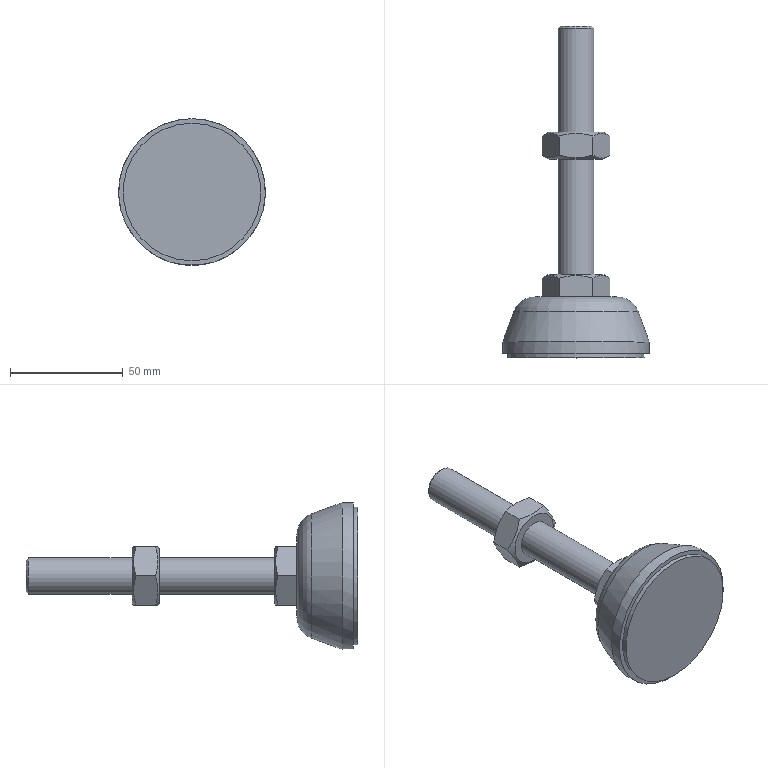Part | STEP file | Foot cup | 2 solids | 32 faces | box 65 x 147 x 65 mm | volume 56921 mm3 | plane 21 | cone 4 | cylinder 4 | torus 3 | commonest cylinder face diameters 16 x2 61 x1 65 x1
STEP:
#1=CARTESIAN_POINT('',(0.,96.,8.));
#2=VERTEX_POINT('',#1);
#3=CARTESIAN_POINT('',(0.,96.,0.));
#4=DIRECTION('',(0.,-1.,0.));
#5=DIRECTION('',(0.,0.,1.));
#6=AXIS2_PLACEMENT_3D('',#3,#4,#5);
#7=CIRCLE('',#6,8.);
#8=EDGE_CURVE('',#2,#2,#7,.T.);
#9=ORIENTED_EDGE('',*,*,#8,.F.);
#10=EDGE_LOOP('',(#9));
#11=FACE_BOUND('',#10,.T.);
#12=CARTESIAN_POINT('',(0.,96.,12.));
#13=VERTEX_POINT('',#12);
#14=CARTESIAN_POINT('',(0.,96.,0.));
#15=DIRECTION('',(0.,1.,0.));
#16=DIRECTION('',(0.,0.,1.));
#17=AXIS2_PLACEMENT_3D('',#14,#15,#16);
#18=CIRCLE('',#17,12.);
#19=EDGE_CURVE('',#13,#13,#18,.T.);
#20=ORIENTED_EDGE('',*,*,#19,.F.);
#21=EDGE_LOOP('',(#20));
#22=FACE_OUTER_BOUND('',#21,.T.);
#23=CARTESIAN_POINT('',(-15.,96.,0.));
#24=DIRECTION('',(0.,1.,0.));
#25=DIRECTION('',(0.,0.,1.));
#26=AXIS2_PLACEMENT_3D('',#23,#24,#25);
#27=PLANE('',#26);
#28=ADVANCED_FACE('',(#11,#22),#27,.F.);
#29=CARTESIAN_POINT('',(0.,45.,-8.));
#30=VERTEX_POINT('',#29);
#31=CARTESIAN_POINT('',(0.,45.,0.));
#32=DIRECTION('',(0.,1.,0.));
#33=DIRECTION('',(0.,0.,-1.));
#34=AXIS2_PLACEMENT_3D('',#31,#32,#33);
#35=CIRCLE('',#34,8.);
#36=EDGE_CURVE('',#30,#30,#35,.T.);
#37=ORIENTED_EDGE('',*,*,#36,.T.);
#38=EDGE_LOOP('',(#37));
#39=FACE_OUTER_BOUND('',#38,.T.);
#40=ORIENTED_EDGE('',*,*,#8,.T.);
#41=EDGE_LOOP('',(#40));
#42=FACE_OUTER_BOUND('',#41,.T.);
#43=CARTESIAN_POINT('',(0.,47.727,0.));
#44=DIRECTION('',(0.,1.,0.));
#45=DIRECTION('',(0.,0.,1.));
#46=AXIS2_PLACEMENT_3D('',#43,#44,#45);
#47=CYLINDRICAL_SURFACE('',#46,8.);
#48=ADVANCED_FACE('',(#39,#42),#47,.T.);
#49=CARTESIAN_POINT('',(0.,35.,18.177));
#50=VERTEX_POINT('',#49);
#51=CARTESIAN_POINT('',(0.,35.,0.));
#52=DIRECTION('',(0.,1.,0.));
#53=DIRECTION('',(0.,0.,1.));
#54=AXIS2_PLACEMENT_3D('',#51,#52,#53);
#55=CIRCLE('',#54,18.177);
#56=EDGE_CURVE('',#50,#50,#55,.T.);
#57=ORIENTED_EDGE('',*,*,#56,.T.);
#58=EDGE_LOOP('',(#57));
#59=FACE_OUTER_BOUND('',#58,.T.);
#60=CARTESIAN_POINT('',(-15.,35.,0.));
#61=VERTEX_POINT('',#60);
#62=CARTESIAN_POINT('',(-7.5,35.,12.99));
#63=VERTEX_POINT('',#62);
#64=CARTESIAN_POINT('',(-7.5,35.,12.99));
#65=DIRECTION('',(0.5,0.,0.866));
#66=VECTOR('',#65,1000.);
#67=LINE('',#64,#66);
#68=EDGE_CURVE('',#61,#63,#67,.T.);
#69=ORIENTED_EDGE('',*,*,#68,.F.);
#70=CARTESIAN_POINT('',(-7.5,35.,-12.99));
#71=VERTEX_POINT('',#70);
#72=CARTESIAN_POINT('',(-15.,35.,0.));
#73=DIRECTION('',(-0.5,0.,0.866));
#74=VECTOR('',#73,1000.);
#75=LINE('',#72,#74);
#76=EDGE_CURVE('',#71,#61,#75,.T.);
#77=ORIENTED_EDGE('',*,*,#76,.F.);
#78=CARTESIAN_POINT('',(7.5,35.,-12.99));
#79=VERTEX_POINT('',#78);
#80=CARTESIAN_POINT('',(-7.5,35.,-12.99));
#81=DIRECTION('',(-1.,0.,0.));
#82=VECTOR('',#81,1000.);
#83=LINE('',#80,#82);
#84=EDGE_CURVE('',#79,#71,#83,.T.);
#85=ORIENTED_EDGE('',*,*,#84,.F.);
#86=CARTESIAN_POINT('',(15.,35.,0.));
#87=VERTEX_POINT('',#86);
#88=CARTESIAN_POINT('',(7.5,35.,-12.99));
#89=DIRECTION('',(-0.5,0.,-0.866));
#90=VECTOR('',#89,1000.);
#91=LINE('',#88,#90);
#92=EDGE_CURVE('',#87,#79,#91,.T.);
#93=ORIENTED_EDGE('',*,*,#92,.F.);
#94=CARTESIAN_POINT('',(7.5,35.,12.99));
#95=VERTEX_POINT('',#94);
#96=CARTESIAN_POINT('',(15.,35.,0.));
#97=DIRECTION('',(0.5,0.,-0.866));
#98=VECTOR('',#97,1000.);
#99=LINE('',#96,#98);
#100=EDGE_CURVE('',#95,#87,#99,.T.);
#101=ORIENTED_EDGE('',*,*,#100,.F.);
#102=CARTESIAN_POINT('',(7.5,35.,12.99));
#103=DIRECTION('',(1.,0.,0.));
#104=VECTOR('',#103,1000.);
#105=LINE('',#102,#104);
#106=EDGE_CURVE('',#63,#95,#105,.T.);
#107=ORIENTED_EDGE('',*,*,#106,.F.);
#108=EDGE_LOOP('',(#69,#77,#85,#93,#101,#107));
#109=FACE_BOUND('',#108,.T.);
#110=CARTESIAN_POINT('',(-25.,35.,0.));
#111=DIRECTION('',(0.,1.,0.));
#112=DIRECTION('',(0.,0.,1.));
#113=AXIS2_PLACEMENT_3D('',#110,#111,#112);
#114=PLANE('',#113);
#115=ADVANCED_FACE('',(#59,#109),#114,.T.);
#116=CARTESIAN_POINT('',(0.,28.582,-27.513));
#117=VERTEX_POINT('',#116);
#118=CARTESIAN_POINT('',(0.,28.582,0.));
#119=DIRECTION('',(0.,-1.,0.));
#120=DIRECTION('',(0.,0.,-1.));
#121=AXIS2_PLACEMENT_3D('',#118,#119,#120);
#122=CIRCLE('',#121,27.513);
#123=EDGE_CURVE('',#117,#117,#122,.T.);
#124=ORIENTED_EDGE('',*,*,#123,.T.);
#125=EDGE_LOOP('',(#124));
#126=FACE_OUTER_BOUND('',#125,.T.);
#127=CARTESIAN_POINT('',(0.,15.,32.5));
#128=VERTEX_POINT('',#127);
#129=CARTESIAN_POINT('',(0.,15.,0.));
#130=DIRECTION('',(0.,1.,0.));
#131=DIRECTION('',(0.,0.,1.));
#132=AXIS2_PLACEMENT_3D('',#129,#130,#131);
#133=CIRCLE('',#132,32.5);
#134=EDGE_CURVE('',#128,#128,#133,.T.);
#135=ORIENTED_EDGE('',*,*,#134,.T.);
#136=EDGE_LOOP('',(#135));
#137=FACE_OUTER_BOUND('',#136,.T.);
#138=CARTESIAN_POINT('',(0.,-150.522,0.));
#139=DIRECTION('',(0.,1.,0.));
#140=DIRECTION('',(0.,0.,1.));
#141=AXIS2_PLACEMENT_3D('',#138,#139,#140);
#142=TOROIDAL_SURFACE('',#141,-439.308,500.);
#143=ADVANCED_FACE('',(#126,#137),#142,.T.);
#144=CARTESIAN_POINT('',(0.,10.,32.5));
#145=VERTEX_POINT('',#144);
#146=CARTESIAN_POINT('',(0.,10.,0.));
#147=DIRECTION('',(0.,1.,0.));
#148=DIRECTION('',(0.,0.,1.));
#149=AXIS2_PLACEMENT_3D('',#146,#147,#148);
#150=CIRCLE('',#149,32.5);
#151=EDGE_CURVE('',#145,#145,#150,.T.);
#152=ORIENTED_EDGE('',*,*,#151,.T.);
#153=EDGE_LOOP('',(#152));
#154=FACE_OUTER_BOUND('',#153,.T.);
#155=ORIENTED_EDGE('',*,*,#134,.F.);
#156=EDGE_LOOP('',(#155));
#157=FACE_OUTER_BOUND('',#156,.T.);
#158=CARTESIAN_POINT('',(0.,47.727,0.));
#159=DIRECTION('',(0.,1.,0.));
#160=DIRECTION('',(0.,0.,1.));
#161=AXIS2_PLACEMENT_3D('',#158,#159,#160);
#162=CYLINDRICAL_SURFACE('',#161,32.5);
#163=ADVANCED_FACE('',(#154,#157),#162,.T.);
#164=CARTESIAN_POINT('',(0.,10.,30.5));
#165=VERTEX_POINT('',#164);
#166=CARTESIAN_POINT('',(0.,10.,0.));
#167=DIRECTION('',(0.,1.,0.));
#168=DIRECTION('',(0.,0.,1.));
#169=AXIS2_PLACEMENT_3D('',#166,#167,#168);
#170=CIRCLE('',#169,30.5);
#171=EDGE_CURVE('',#165,#165,#170,.T.);
#172=ORIENTED_EDGE('',*,*,#171,.T.);
#173=EDGE_LOOP('',(#172));
#174=FACE_BOUND('',#173,.T.);
#175=ORIENTED_EDGE('',*,*,#151,.F.);
#176=EDGE_LOOP('',(#175));
#177=FACE_OUTER_BOUND('',#176,.T.);
#178=CARTESIAN_POINT('',(-30.5,10.,0.));
#179=DIRECTION('',(0.,-1.,0.));
#180=DIRECTION('',(0.,0.,-1.));
#181=AXIS2_PLACEMENT_3D('',#178,#179,#180);
#182=PLANE('',#181);
#183=ADVANCED_FACE('',(#174,#177),#182,.T.);
#184=CARTESIAN_POINT('',(0.,32.,22.398));
#185=VERTEX_POINT('',#184);
#186=CARTESIAN_POINT('',(0.,32.,0.));
#187=DIRECTION('',(0.,1.,0.));
#188=DIRECTION('',(0.,0.,1.));
#189=AXIS2_PLACEMENT_3D('',#186,#187,#188);
#190=CIRCLE('',#189,22.398);
#191=EDGE_CURVE('',#185,#185,#190,.T.);
#192=ORIENTED_EDGE('',*,*,#191,.T.);
#193=EDGE_LOOP('',(#192));
#194=FACE_OUTER_BOUND('',#193,.T.);
#195=ORIENTED_EDGE('',*,*,#171,.F.);
#196=EDGE_LOOP('',(#195));
#197=FACE_OUTER_BOUND('',#196,.T.);
#198=CARTESIAN_POINT('',(0.,-150.522,0.));
#199=DIRECTION('',(0.,1.,0.));
#200=DIRECTION('',(0.,0.,1.));
#201=AXIS2_PLACEMENT_3D('',#198,#199,#200);
#202=TOROIDAL_SURFACE('',#201,-439.308,496.474);
#203=ADVANCED_FACE('',(#194,#197),#202,.F.);
#204=ORIENTED_EDGE('',*,*,#191,.F.);
#205=EDGE_LOOP('',(#204));
#206=FACE_OUTER_BOUND('',#205,.T.);
#207=CARTESIAN_POINT('',(-22.398,32.,0.));
#208=DIRECTION('',(0.,-1.,0.));
#209=DIRECTION('',(0.,0.,-1.));
#210=AXIS2_PLACEMENT_3D('',#207,#208,#209);
#211=PLANE('',#210);
#212=ADVANCED_FACE('',(#206),#211,.T.);
#213=CARTESIAN_POINT('',(-15.,43.268,0.));
#214=VERTEX_POINT('',#213);
#215=CARTESIAN_POINT('',(-15.,45.,0.));
#216=DIRECTION('',(0.,-1.,0.));
#217=VECTOR('',#216,1000.);
#218=LINE('',#215,#217);
#219=EDGE_CURVE('',#214,#61,#218,.T.);
#220=ORIENTED_EDGE('',*,*,#219,.F.);
#221=CARTESIAN_POINT('',(-7.5,43.268,-12.99));
#222=VERTEX_POINT('',#221);
#223=CARTESIAN_POINT('',(-15.,43.268,0.));
#224=CARTESIAN_POINT('',(-14.388,43.621,-1.061));
#225=CARTESIAN_POINT('',(-13.771,43.913,-2.129));
#226=CARTESIAN_POINT('',(-12.525,44.316,-4.288));
#227=CARTESIAN_POINT('',(-11.895,44.427,-5.378));
#228=CARTESIAN_POINT('',(-10.938,44.429,-7.035));
#229=CARTESIAN_POINT('',(-10.618,44.401,-7.59));
#230=CARTESIAN_POINT('',(-9.984,44.296,-8.687));
#231=CARTESIAN_POINT('',(-9.67,44.217,-9.232));
#232=CARTESIAN_POINT('',(-8.731,43.914,-10.858));
#233=CARTESIAN_POINT('',(-8.113,43.622,-11.929));
#234=CARTESIAN_POINT('',(-7.5,43.268,-12.99));
#235=B_SPLINE_CURVE_WITH_KNOTS('',3,(#223,#224,#225,#226,#227,#228,#229,#230,#231,#232,#233,#234),.UNSPECIFIED.,.F.,.F.,(4,2,2,2,2,4),(0.000000238,0.003788,0.007575,0.009468,0.01136,0.01515),.UNSPECIFIED.);
#236=EDGE_CURVE('',#214,#222,#235,.T.);
#237=ORIENTED_EDGE('',*,*,#236,.T.);
#238=CARTESIAN_POINT('',(-7.5,45.,-12.99));
#239=DIRECTION('',(0.,-1.,0.));
#240=VECTOR('',#239,1000.);
#241=LINE('',#238,#240);
#242=EDGE_CURVE('',#222,#71,#241,.T.);
#243=ORIENTED_EDGE('',*,*,#242,.T.);
#244=ORIENTED_EDGE('',*,*,#76,.T.);
#245=EDGE_LOOP('',(#220,#237,#243,#244));
#246=FACE_OUTER_BOUND('',#245,.T.);
#247=CARTESIAN_POINT('',(-15.,45.,0.));
#248=DIRECTION('',(0.866,0.,0.5));
#249=DIRECTION('',(0.5,0.,-0.866));
#250=AXIS2_PLACEMENT_3D('',#247,#248,#249);
#251=PLANE('',#250);
#252=ADVANCED_FACE('',(#246),#251,.F.);
#253=CARTESIAN_POINT('',(-7.5,43.268,12.99));
#254=VERTEX_POINT('',#253);
#255=CARTESIAN_POINT('',(-7.5,45.,12.99));
#256=DIRECTION('',(0.,-1.,0.));
#257=VECTOR('',#256,1000.);
#258=LINE('',#255,#257);
#259=EDGE_CURVE('',#254,#63,#258,.T.);
#260=ORIENTED_EDGE('',*,*,#259,.F.);
#261=CARTESIAN_POINT('',(-7.5,43.268,12.99));
#262=CARTESIAN_POINT('',(-8.112,43.621,11.93));
#263=CARTESIAN_POINT('',(-8.729,43.913,10.862));
#264=CARTESIAN_POINT('',(-9.975,44.316,8.703));
#265=CARTESIAN_POINT('',(-10.605,44.427,7.612));
#266=CARTESIAN_POINT('',(-11.562,44.429,5.955));
#267=CARTESIAN_POINT('',(-11.882,44.401,5.401));
#268=CARTESIAN_POINT('',(-12.516,44.296,4.303));
#269=CARTESIAN_POINT('',(-12.83,44.217,3.758));
#270=CARTESIAN_POINT('',(-13.769,43.914,2.133));
#271=CARTESIAN_POINT('',(-14.387,43.622,1.062));
#272=CARTESIAN_POINT('',(-15.,43.268,0.));
#273=B_SPLINE_CURVE_WITH_KNOTS('',3,(#261,#262,#263,#264,#265,#266,#267,#268,#269,#270,#271,#272),.UNSPECIFIED.,.F.,.F.,(4,2,2,2,2,4),(0.000000238,0.003788,0.007575,0.009468,0.01136,0.01515),.UNSPECIFIED.);
#274=EDGE_CURVE('',#254,#214,#273,.T.);
#275=ORIENTED_EDGE('',*,*,#274,.T.);
#276=ORIENTED_EDGE('',*,*,#219,.T.);
#277=ORIENTED_EDGE('',*,*,#68,.T.);
#278=EDGE_LOOP('',(#260,#275,#276,#277));
#279=FACE_OUTER_BOUND('',#278,.T.);
#280=CARTESIAN_POINT('',(-7.5,45.,12.99));
#281=DIRECTION('',(0.866,0.,-0.5));
#282=DIRECTION('',(-0.5,0.,-0.866));
#283=AXIS2_PLACEMENT_3D('',#280,#281,#282);
#284=PLANE('',#283);
#285=ADVANCED_FACE('',(#279),#284,.F.);
#286=CARTESIAN_POINT('',(7.5,43.268,12.99));
#287=VERTEX_POINT('',#286);
#288=CARTESIAN_POINT('',(7.5,45.,12.99));
#289=DIRECTION('',(0.,-1.,0.));
#290=VECTOR('',#289,1000.);
#291=LINE('',#288,#290);
#292=EDGE_CURVE('',#287,#95,#291,.T.);
#293=ORIENTED_EDGE('',*,*,#292,.F.);
#294=CARTESIAN_POINT('',(7.5,43.268,12.99));
#295=CARTESIAN_POINT('',(6.288,43.618,12.99));
#296=CARTESIAN_POINT('',(5.059,43.909,12.99));
#297=CARTESIAN_POINT('',(3.181,44.214,12.99));
#298=CARTESIAN_POINT('',(2.547,44.294,12.99));
#299=CARTESIAN_POINT('',(1.272,44.401,12.99));
#300=CARTESIAN_POINT('',(0.6359,44.428,12.99));
#301=CARTESIAN_POINT('',(-1.265,44.428,12.99));
#302=CARTESIAN_POINT('',(-2.525,44.319,12.99));
#303=CARTESIAN_POINT('',(-4.404,44.017,12.99));
#304=CARTESIAN_POINT('',(-5.029,43.892,12.99));
#305=CARTESIAN_POINT('',(-6.275,43.606,12.99));
#306=CARTESIAN_POINT('',(-6.89,43.444,12.99));
#307=CARTESIAN_POINT('',(-7.5,43.268,12.99));
#308=B_SPLINE_CURVE_WITH_KNOTS('',3,(#294,#295,#296,#297,#298,#299,#300,#301,#302,#303,#304,#305,#306,#307),.UNSPECIFIED.,.F.,.F.,(4,2,2,2,2,2,4),(0.005592,0.009378,0.01127,0.01316,0.01695,0.01884,0.02073),.UNSPECIFIED.);
#309=EDGE_CURVE('',#287,#254,#308,.T.);
#310=ORIENTED_EDGE('',*,*,#309,.T.);
#311=ORIENTED_EDGE('',*,*,#259,.T.);
#312=ORIENTED_EDGE('',*,*,#106,.T.);
#313=EDGE_LOOP('',(#293,#310,#311,#312));
#314=FACE_OUTER_BOUND('',#313,.T.);
#315=CARTESIAN_POINT('',(7.5,45.,12.99));
#316=DIRECTION('',(0.,0.,-1.));
#317=DIRECTION('',(-1.,0.,0.));
#318=AXIS2_PLACEMENT_3D('',#315,#316,#317);
#319=PLANE('',#318);
#320=ADVANCED_FACE('',(#314),#319,.F.);
#321=CARTESIAN_POINT('',(15.,43.268,0.));
#322=VERTEX_POINT('',#321);
#323=CARTESIAN_POINT('',(15.,45.,0.));
#324=DIRECTION('',(0.,-1.,0.));
#325=VECTOR('',#324,1000.);
#326=LINE('',#323,#325);
#327=EDGE_CURVE('',#322,#87,#326,.T.);
#328=ORIENTED_EDGE('',*,*,#327,.F.);
#329=CARTESIAN_POINT('',(15.,43.268,0.));
#330=CARTESIAN_POINT('',(14.388,43.621,1.061));
#331=CARTESIAN_POINT('',(13.771,43.913,2.129));
#332=CARTESIAN_POINT('',(12.525,44.316,4.288));
#333=CARTESIAN_POINT('',(11.895,44.427,5.378));
#334=CARTESIAN_POINT('',(10.938,44.429,7.035));
#335=CARTESIAN_POINT('',(10.618,44.401,7.59));
#336=CARTESIAN_POINT('',(9.984,44.296,8.687));
#337=CARTESIAN_POINT('',(9.67,44.217,9.232));
#338=CARTESIAN_POINT('',(8.731,43.914,10.858));
#339=CARTESIAN_POINT('',(8.113,43.622,11.929));
#340=CARTESIAN_POINT('',(7.5,43.268,12.99));
#341=B_SPLINE_CURVE_WITH_KNOTS('',3,(#329,#330,#331,#332,#333,#334,#335,#336,#337,#338,#339,#340),.UNSPECIFIED.,.F.,.F.,(4,2,2,2,2,4),(0.000000238,0.003788,0.007575,0.009468,0.01136,0.01515),.UNSPECIFIED.);
#342=EDGE_CURVE('',#322,#287,#341,.T.);
#343=ORIENTED_EDGE('',*,*,#342,.T.);
#344=ORIENTED_EDGE('',*,*,#292,.T.);
#345=ORIENTED_EDGE('',*,*,#100,.T.);
#346=EDGE_LOOP('',(#328,#343,#344,#345));
#347=FACE_OUTER_BOUND('',#346,.T.);
#348=CARTESIAN_POINT('',(15.,45.,0.));
#349=DIRECTION('',(-0.866,0.,-0.5));
#350=DIRECTION('',(-0.5,0.,0.866));
#351=AXIS2_PLACEMENT_3D('',#348,#349,#350);
#352=PLANE('',#351);
#353=ADVANCED_FACE('',(#347),#352,.F.);
#354=CARTESIAN_POINT('',(7.5,43.268,-12.99));
#355=VERTEX_POINT('',#354);
#356=CARTESIAN_POINT('',(7.5,45.,-12.99));
#357=DIRECTION('',(0.,-1.,0.));
#358=VECTOR('',#357,1000.);
#359=LINE('',#356,#358);
#360=EDGE_CURVE('',#355,#79,#359,.T.);
#361=ORIENTED_EDGE('',*,*,#360,.F.);
#362=CARTESIAN_POINT('',(7.5,43.268,-12.99));
#363=CARTESIAN_POINT('',(8.112,43.621,-11.93));
#364=CARTESIAN_POINT('',(8.729,43.913,-10.862));
#365=CARTESIAN_POINT('',(9.975,44.316,-8.703));
#366=CARTESIAN_POINT('',(10.605,44.427,-7.612));
#367=CARTESIAN_POINT('',(11.562,44.429,-5.955));
#368=CARTESIAN_POINT('',(11.882,44.401,-5.401));
#369=CARTESIAN_POINT('',(12.516,44.296,-4.303));
#370=CARTESIAN_POINT('',(12.83,44.217,-3.758));
#371=CARTESIAN_POINT('',(13.769,43.914,-2.133));
#372=CARTESIAN_POINT('',(14.387,43.622,-1.062));
#373=CARTESIAN_POINT('',(15.,43.268,0.));
#374=B_SPLINE_CURVE_WITH_KNOTS('',3,(#362,#363,#364,#365,#366,#367,#368,#369,#370,#371,#372,#373),.UNSPECIFIED.,.F.,.F.,(4,2,2,2,2,4),(0.000000238,0.003788,0.007575,0.009468,0.01136,0.01515),.UNSPECIFIED.);
#375=EDGE_CURVE('',#355,#322,#374,.T.);
#376=ORIENTED_EDGE('',*,*,#375,.T.);
#377=ORIENTED_EDGE('',*,*,#327,.T.);
#378=ORIENTED_EDGE('',*,*,#92,.T.);
#379=EDGE_LOOP('',(#361,#376,#377,#378));
#380=FACE_OUTER_BOUND('',#379,.T.);
#381=CARTESIAN_POINT('',(7.5,45.,-12.99));
#382=DIRECTION('',(-0.866,0.,0.5));
#383=DIRECTION('',(0.5,0.,0.866));
#384=AXIS2_PLACEMENT_3D('',#381,#382,#383);
#385=PLANE('',#384);
#386=ADVANCED_FACE('',(#380),#385,.F.);
#387=ORIENTED_EDGE('',*,*,#242,.F.);
#388=CARTESIAN_POINT('',(-7.5,43.268,-12.99));
#389=CARTESIAN_POINT('',(-6.89,43.444,-12.99));
#390=CARTESIAN_POINT('',(-6.275,43.606,-12.99));
#391=CARTESIAN_POINT('',(-5.029,43.892,-12.99));
#392=CARTESIAN_POINT('',(-4.404,44.017,-12.99));
#393=CARTESIAN_POINT('',(-2.525,44.319,-12.99));
#394=CARTESIAN_POINT('',(-1.265,44.428,-12.99));
#395=CARTESIAN_POINT('',(0.6359,44.428,-12.99));
#396=CARTESIAN_POINT('',(1.272,44.401,-12.99));
#397=CARTESIAN_POINT('',(2.547,44.294,-12.99));
#398=CARTESIAN_POINT('',(3.181,44.214,-12.99));
#399=CARTESIAN_POINT('',(5.059,43.909,-12.99));
#400=CARTESIAN_POINT('',(6.288,43.618,-12.99));
#401=CARTESIAN_POINT('',(7.5,43.268,-12.99));
#402=B_SPLINE_CURVE_WITH_KNOTS('',3,(#388,#389,#390,#391,#392,#393,#394,#395,#396,#397,#398,#399,#400,#401),.UNSPECIFIED.,.F.,.F.,(4,2,2,2,2,2,4),(0.01329,0.01519,0.01709,0.02088,0.02278,0.02468,0.02847),.UNSPECIFIED.);
#403=EDGE_CURVE('',#222,#355,#402,.T.);
#404=ORIENTED_EDGE('',*,*,#403,.T.);
#405=ORIENTED_EDGE('',*,*,#360,.T.);
#406=ORIENTED_EDGE('',*,*,#84,.T.);
#407=EDGE_LOOP('',(#387,#404,#405,#406));
#408=FACE_OUTER_BOUND('',#407,.T.);
#409=CARTESIAN_POINT('',(-7.5,45.,-12.99));
#410=DIRECTION('',(0.,0.,1.));
#411=DIRECTION('',(1.,0.,0.));
#412=AXIS2_PLACEMENT_3D('',#409,#410,#411);
#413=PLANE('',#412);
#414=ADVANCED_FACE('',(#408),#413,.F.);
#415=CARTESIAN_POINT('',(0.,45.,-12.));
#416=VERTEX_POINT('',#415);
#417=CARTESIAN_POINT('',(0.,45.,0.));
#418=DIRECTION('',(0.,-1.,0.));
#419=DIRECTION('',(0.,0.,-1.));
#420=AXIS2_PLACEMENT_3D('',#417,#418,#419);
#421=CIRCLE('',#420,12.);
#422=EDGE_CURVE('',#416,#416,#421,.T.);
#423=ORIENTED_EDGE('',*,*,#422,.T.);
#424=EDGE_LOOP('',(#423));
#425=FACE_BOUND('',#424,.T.);
#426=ORIENTED_EDGE('',*,*,#274,.F.);
#427=ORIENTED_EDGE('',*,*,#309,.F.);
#428=ORIENTED_EDGE('',*,*,#342,.F.);
#429=ORIENTED_EDGE('',*,*,#375,.F.);
#430=ORIENTED_EDGE('',*,*,#403,.F.);
#431=ORIENTED_EDGE('',*,*,#236,.F.);
#432=EDGE_LOOP('',(#426,#427,#428,#429,#430,#431));
#433=FACE_OUTER_BOUND('',#432,.T.);
#434=CARTESIAN_POINT('',(0.,45.,0.));
#435=DIRECTION('',(0.,-1.,0.));
#436=DIRECTION('',(0.,0.,-1.));
#437=AXIS2_PLACEMENT_3D('',#434,#435,#436);
#438=CONICAL_SURFACE('',#437,12.,1.047);
#439=ADVANCED_FACE('',(#425,#433),#438,.T.);
#440=ORIENTED_EDGE('',*,*,#422,.F.);
#441=EDGE_LOOP('',(#440));
#442=FACE_OUTER_BOUND('',#441,.T.);
#443=ORIENTED_EDGE('',*,*,#36,.F.);
#444=EDGE_LOOP('',(#443));
#445=FACE_BOUND('',#444,.T.);
#446=CARTESIAN_POINT('',(0.,45.,-25.981));
#447=DIRECTION('',(0.,-1.,0.));
#448=DIRECTION('',(0.,0.,-1.));
#449=AXIS2_PLACEMENT_3D('',#446,#447,#448);
#450=PLANE('',#449);
#451=ADVANCED_FACE('',(#442,#445),#450,.F.);
#452=ORIENTED_EDGE('',*,*,#19,.T.);
#453=EDGE_LOOP('',(#452));
#454=FACE_BOUND('',#453,.T.);
#455=CARTESIAN_POINT('',(-15.,97.732,0.));
#456=VERTEX_POINT('',#455);
#457=CARTESIAN_POINT('',(-7.5,97.732,-12.99));
#458=VERTEX_POINT('',#457);
#459=CARTESIAN_POINT('',(-15.,97.732,0.));
#460=CARTESIAN_POINT('',(-14.388,97.379,-1.061));
#461=CARTESIAN_POINT('',(-13.771,97.087,-2.129));
#462=CARTESIAN_POINT('',(-12.525,96.684,-4.288));
#463=CARTESIAN_POINT('',(-11.895,96.573,-5.378));
#464=CARTESIAN_POINT('',(-10.938,96.571,-7.035));
#465=CARTESIAN_POINT('',(-10.618,96.599,-7.59));
#466=CARTESIAN_POINT('',(-9.984,96.704,-8.687));
#467=CARTESIAN_POINT('',(-9.67,96.783,-9.232));
#468=CARTESIAN_POINT('',(-8.731,97.086,-10.858));
#469=CARTESIAN_POINT('',(-8.113,97.378,-11.929));
#470=CARTESIAN_POINT('',(-7.5,97.732,-12.99));
#471=B_SPLINE_CURVE_WITH_KNOTS('',3,(#459,#460,#461,#462,#463,#464,#465,#466,#467,#468,#469,#470),.UNSPECIFIED.,.F.,.F.,(4,2,2,2,2,4),(0.000000238,0.003788,0.007575,0.009468,0.01136,0.01515),.UNSPECIFIED.);
#472=EDGE_CURVE('',#456,#458,#471,.T.);
#473=ORIENTED_EDGE('',*,*,#472,.T.);
#474=CARTESIAN_POINT('',(7.5,97.732,-12.99));
#475=VERTEX_POINT('',#474);
#476=CARTESIAN_POINT('',(-7.5,97.732,-12.99));
#477=CARTESIAN_POINT('',(-6.89,97.556,-12.99));
#478=CARTESIAN_POINT('',(-6.275,97.394,-12.99));
#479=CARTESIAN_POINT('',(-5.029,97.108,-12.99));
#480=CARTESIAN_POINT('',(-4.404,96.983,-12.99));
#481=CARTESIAN_POINT('',(-2.525,96.681,-12.99));
#482=CARTESIAN_POINT('',(-1.265,96.572,-12.99));
#483=CARTESIAN_POINT('',(0.6359,96.572,-12.99));
#484=CARTESIAN_POINT('',(1.272,96.599,-12.99));
#485=CARTESIAN_POINT('',(2.547,96.706,-12.99));
#486=CARTESIAN_POINT('',(3.181,96.786,-12.99));
#487=CARTESIAN_POINT('',(5.059,97.091,-12.99));
#488=CARTESIAN_POINT('',(6.288,97.382,-12.99));
#489=CARTESIAN_POINT('',(7.5,97.732,-12.99));
#490=B_SPLINE_CURVE_WITH_KNOTS('',3,(#476,#477,#478,#479,#480,#481,#482,#483,#484,#485,#486,#487,#488,#489),.UNSPECIFIED.,.F.,.F.,(4,2,2,2,2,2,4),(0.01329,0.01519,0.01709,0.02088,0.02278,0.02468,0.02847),.UNSPECIFIED.);
#491=EDGE_CURVE('',#458,#475,#490,.T.);
#492=ORIENTED_EDGE('',*,*,#491,.T.);
#493=CARTESIAN_POINT('',(15.,97.732,0.));
#494=VERTEX_POINT('',#493);
#495=CARTESIAN_POINT('',(7.5,97.732,-12.99));
#496=CARTESIAN_POINT('',(8.112,97.379,-11.93));
#497=CARTESIAN_POINT('',(8.729,97.087,-10.862));
#498=CARTESIAN_POINT('',(9.975,96.684,-8.703));
#499=CARTESIAN_POINT('',(10.605,96.573,-7.612));
#500=CARTESIAN_POINT('',(11.562,96.571,-5.955));
#501=CARTESIAN_POINT('',(11.882,96.599,-5.401));
#502=CARTESIAN_POINT('',(12.516,96.704,-4.303));
#503=CARTESIAN_POINT('',(12.83,96.783,-3.758));
#504=CARTESIAN_POINT('',(13.769,97.086,-2.133));
#505=CARTESIAN_POINT('',(14.387,97.378,-1.062));
#506=CARTESIAN_POINT('',(15.,97.732,0.));
#507=B_SPLINE_CURVE_WITH_KNOTS('',3,(#495,#496,#497,#498,#499,#500,#501,#502,#503,#504,#505,#506),.UNSPECIFIED.,.F.,.F.,(4,2,2,2,2,4),(0.000000238,0.003788,0.007575,0.009468,0.01136,0.01515),.UNSPECIFIED.);
#508=EDGE_CURVE('',#475,#494,#507,.T.);
#509=ORIENTED_EDGE('',*,*,#508,.T.);
#510=CARTESIAN_POINT('',(7.5,97.732,12.99));
#511=VERTEX_POINT('',#510);
#512=CARTESIAN_POINT('',(15.,97.732,0.));
#513=CARTESIAN_POINT('',(14.388,97.379,1.061));
#514=CARTESIAN_POINT('',(13.771,97.087,2.129));
#515=CARTESIAN_POINT('',(12.525,96.684,4.288));
#516=CARTESIAN_POINT('',(11.895,96.573,5.378));
#517=CARTESIAN_POINT('',(10.938,96.571,7.035));
#518=CARTESIAN_POINT('',(10.618,96.599,7.59));
#519=CARTESIAN_POINT('',(9.984,96.704,8.687));
#520=CARTESIAN_POINT('',(9.67,96.783,9.232));
#521=CARTESIAN_POINT('',(8.731,97.086,10.858));
#522=CARTESIAN_POINT('',(8.113,97.378,11.929));
#523=CARTESIAN_POINT('',(7.5,97.732,12.99));
#524=B_SPLINE_CURVE_WITH_KNOTS('',3,(#512,#513,#514,#515,#516,#517,#518,#519,#520,#521,#522,#523),.UNSPECIFIED.,.F.,.F.,(4,2,2,2,2,4),(0.000000238,0.003788,0.007575,0.009468,0.01136,0.01515),.UNSPECIFIED.);
#525=EDGE_CURVE('',#494,#511,#524,.T.);
#526=ORIENTED_EDGE('',*,*,#525,.T.);
#527=CARTESIAN_POINT('',(-7.5,97.732,12.99));
#528=VERTEX_POINT('',#527);
#529=CARTESIAN_POINT('',(7.5,97.732,12.99));
#530=CARTESIAN_POINT('',(6.288,97.382,12.99));
#531=CARTESIAN_POINT('',(5.059,97.091,12.99));
#532=CARTESIAN_POINT('',(3.181,96.786,12.99));
#533=CARTESIAN_POINT('',(2.547,96.706,12.99));
#534=CARTESIAN_POINT('',(1.272,96.599,12.99));
#535=CARTESIAN_POINT('',(0.6359,96.572,12.99));
#536=CARTESIAN_POINT('',(-1.265,96.572,12.99));
#537=CARTESIAN_POINT('',(-2.525,96.681,12.99));
#538=CARTESIAN_POINT('',(-4.404,96.983,12.99));
#539=CARTESIAN_POINT('',(-5.029,97.108,12.99));
#540=CARTESIAN_POINT('',(-6.275,97.394,12.99));
#541=CARTESIAN_POINT('',(-6.89,97.556,12.99));
#542=CARTESIAN_POINT('',(-7.5,97.732,12.99));
#543=B_SPLINE_CURVE_WITH_KNOTS('',3,(#529,#530,#531,#532,#533,#534,#535,#536,#537,#538,#539,#540,#541,#542),.UNSPECIFIED.,.F.,.F.,(4,2,2,2,2,2,4),(0.005592,0.009378,0.01127,0.01316,0.01695,0.01884,0.02073),.UNSPECIFIED.);
#544=EDGE_CURVE('',#511,#528,#543,.T.);
#545=ORIENTED_EDGE('',*,*,#544,.T.);
#546=CARTESIAN_POINT('',(-7.5,97.732,12.99));
#547=CARTESIAN_POINT('',(-8.112,97.379,11.93));
#548=CARTESIAN_POINT('',(-8.729,97.087,10.862));
#549=CARTESIAN_POINT('',(-9.975,96.684,8.703));
#550=CARTESIAN_POINT('',(-10.605,96.573,7.612));
#551=CARTESIAN_POINT('',(-11.562,96.571,5.955));
#552=CARTESIAN_POINT('',(-11.882,96.599,5.401));
#553=CARTESIAN_POINT('',(-12.516,96.704,4.303));
#554=CARTESIAN_POINT('',(-12.83,96.783,3.758));
#555=CARTESIAN_POINT('',(-13.769,97.086,2.133));
#556=CARTESIAN_POINT('',(-14.387,97.378,1.062));
#557=CARTESIAN_POINT('',(-15.,97.732,0.));
#558=B_SPLINE_CURVE_WITH_KNOTS('',3,(#546,#547,#548,#549,#550,#551,#552,#553,#554,#555,#556,#557),.UNSPECIFIED.,.F.,.F.,(4,2,2,2,2,4),(0.000000238,0.003788,0.007575,0.009468,0.01136,0.01515),.UNSPECIFIED.);
#559=EDGE_CURVE('',#528,#456,#558,.T.);
#560=ORIENTED_EDGE('',*,*,#559,.T.);
#561=EDGE_LOOP('',(#473,#492,#509,#526,#545,#560));
#562=FACE_OUTER_BOUND('',#561,.T.);
#563=CARTESIAN_POINT('',(0.,97.732,0.));
#564=DIRECTION('',(0.,1.,0.));
#565=DIRECTION('',(0.,0.,1.));
#566=AXIS2_PLACEMENT_3D('',#563,#564,#565);
#567=CONICAL_SURFACE('',#566,15.,1.047);
#568=ADVANCED_FACE('',(#454,#562),#567,.T.);
#569=CARTESIAN_POINT('',(0.,155.,7.));
#570=VERTEX_POINT('',#569);
#571=CARTESIAN_POINT('',(0.,155.,0.));
#572=DIRECTION('',(0.,1.,0.));
#573=DIRECTION('',(0.,0.,1.));
#574=AXIS2_PLACEMENT_3D('',#571,#572,#573);
#575=CIRCLE('',#574,7.);
#576=EDGE_CURVE('',#570,#570,#575,.T.);
#577=ORIENTED_EDGE('',*,*,#576,.T.);
#578=EDGE_LOOP('',(#577));
#579=FACE_OUTER_BOUND('',#578,.T.);
#580=CARTESIAN_POINT('',(-8.,155.,0.));
#581=DIRECTION('',(0.,1.,0.));
#582=DIRECTION('',(0.,0.,1.));
#583=AXIS2_PLACEMENT_3D('',#580,#581,#582);
#584=PLANE('',#583);
#585=ADVANCED_FACE('',(#579),#584,.T.);
#586=CARTESIAN_POINT('',(0.,154.,8.));
#587=VERTEX_POINT('',#586);
#588=CARTESIAN_POINT('',(0.,154.,0.));
#589=DIRECTION('',(0.,-1.,0.));
#590=DIRECTION('',(0.,0.,1.));
#591=AXIS2_PLACEMENT_3D('',#588,#589,#590);
#592=CIRCLE('',#591,8.);
#593=EDGE_CURVE('',#587,#587,#592,.T.);
#594=ORIENTED_EDGE('',*,*,#593,.F.);
#595=EDGE_LOOP('',(#594));
#596=FACE_OUTER_BOUND('',#595,.T.);
#597=ORIENTED_EDGE('',*,*,#576,.F.);
#598=EDGE_LOOP('',(#597));
#599=FACE_BOUND('',#598,.T.);
#600=CARTESIAN_POINT('',(0.,155.,0.));
#601=DIRECTION('',(0.,-1.,0.));
#602=DIRECTION('',(0.,0.,-1.));
#603=AXIS2_PLACEMENT_3D('',#600,#601,#602);
#604=CONICAL_SURFACE('',#603,7.,0.7854);
#605=ADVANCED_FACE('',(#596,#599),#604,.T.);
#606=CARTESIAN_POINT('',(0.,108.,8.));
#607=VERTEX_POINT('',#606);
#608=CARTESIAN_POINT('',(0.,108.,0.));
#609=DIRECTION('',(0.,-1.,0.));
#610=DIRECTION('',(0.,0.,1.));
#611=AXIS2_PLACEMENT_3D('',#608,#609,#610);
#612=CIRCLE('',#611,8.);
#613=EDGE_CURVE('',#607,#607,#612,.T.);
#614=ORIENTED_EDGE('',*,*,#613,.F.);
#615=EDGE_LOOP('',(#614));
#616=FACE_OUTER_BOUND('',#615,.T.);
#617=ORIENTED_EDGE('',*,*,#593,.T.);
#618=EDGE_LOOP('',(#617));
#619=FACE_OUTER_BOUND('',#618,.T.);
#620=CARTESIAN_POINT('',(0.,47.727,0.));
#621=DIRECTION('',(0.,1.,0.));
#622=DIRECTION('',(0.,0.,1.));
#623=AXIS2_PLACEMENT_3D('',#620,#621,#622);
#624=CYLINDRICAL_SURFACE('',#623,8.);
#625=ADVANCED_FACE('',(#616,#619),#624,.T.);
#626=ORIENTED_EDGE('',*,*,#613,.T.);
#627=EDGE_LOOP('',(#626));
#628=FACE_BOUND('',#627,.T.);
#629=CARTESIAN_POINT('',(0.,108.,12.));
#630=VERTEX_POINT('',#629);
#631=CARTESIAN_POINT('',(0.,108.,0.));
#632=DIRECTION('',(0.,1.,0.));
#633=DIRECTION('',(0.,0.,1.));
#634=AXIS2_PLACEMENT_3D('',#631,#632,#633);
#635=CIRCLE('',#634,12.);
#636=EDGE_CURVE('',#630,#630,#635,.T.);
#637=ORIENTED_EDGE('',*,*,#636,.T.);
#638=EDGE_LOOP('',(#637));
#639=FACE_OUTER_BOUND('',#638,.T.);
#640=CARTESIAN_POINT('',(-15.,108.,0.));
#641=DIRECTION('',(0.,1.,0.));
#642=DIRECTION('',(0.,0.,1.));
#643=AXIS2_PLACEMENT_3D('',#640,#641,#642);
#644=PLANE('',#643);
#645=ADVANCED_FACE('',(#628,#639),#644,.T.);
#646=ORIENTED_EDGE('',*,*,#636,.F.);
#647=EDGE_LOOP('',(#646));
#648=FACE_BOUND('',#647,.T.);
#649=CARTESIAN_POINT('',(-7.5,106.268,-12.99));
#650=VERTEX_POINT('',#649);
#651=CARTESIAN_POINT('',(-15.,106.268,0.));
#652=VERTEX_POINT('',#651);
#653=CARTESIAN_POINT('',(-7.5,106.268,-12.99));
#654=CARTESIAN_POINT('',(-8.112,106.621,-11.93));
#655=CARTESIAN_POINT('',(-8.729,106.913,-10.862));
#656=CARTESIAN_POINT('',(-9.975,107.316,-8.703));
#657=CARTESIAN_POINT('',(-10.605,107.427,-7.612));
#658=CARTESIAN_POINT('',(-11.562,107.429,-5.955));
#659=CARTESIAN_POINT('',(-11.882,107.401,-5.401));
#660=CARTESIAN_POINT('',(-12.516,107.296,-4.303));
#661=CARTESIAN_POINT('',(-12.83,107.217,-3.758));
#662=CARTESIAN_POINT('',(-13.769,106.914,-2.133));
#663=CARTESIAN_POINT('',(-14.387,106.622,-1.062));
#664=CARTESIAN_POINT('',(-15.,106.268,0.));
#665=B_SPLINE_CURVE_WITH_KNOTS('',3,(#653,#654,#655,#656,#657,#658,#659,#660,#661,#662,#663,#664),.UNSPECIFIED.,.F.,.F.,(4,2,2,2,2,4),(0.000000238,0.003788,0.007575,0.009468,0.01136,0.01515),.UNSPECIFIED.);
#666=EDGE_CURVE('',#650,#652,#665,.T.);
#667=ORIENTED_EDGE('',*,*,#666,.T.);
#668=CARTESIAN_POINT('',(-7.5,106.268,12.99));
#669=VERTEX_POINT('',#668);
#670=CARTESIAN_POINT('',(-15.,106.268,0.));
#671=CARTESIAN_POINT('',(-14.388,106.621,1.061));
#672=CARTESIAN_POINT('',(-13.771,106.913,2.129));
#673=CARTESIAN_POINT('',(-12.525,107.316,4.288));
#674=CARTESIAN_POINT('',(-11.895,107.427,5.378));
#675=CARTESIAN_POINT('',(-10.938,107.429,7.035));
#676=CARTESIAN_POINT('',(-10.618,107.401,7.59));
#677=CARTESIAN_POINT('',(-9.984,107.296,8.687));
#678=CARTESIAN_POINT('',(-9.67,107.217,9.232));
#679=CARTESIAN_POINT('',(-8.731,106.914,10.858));
#680=CARTESIAN_POINT('',(-8.113,106.622,11.929));
#681=CARTESIAN_POINT('',(-7.5,106.268,12.99));
#682=B_SPLINE_CURVE_WITH_KNOTS('',3,(#670,#671,#672,#673,#674,#675,#676,#677,#678,#679,#680,#681),.UNSPECIFIED.,.F.,.F.,(4,2,2,2,2,4),(0.000000238,0.003788,0.007575,0.009468,0.01136,0.01515),.UNSPECIFIED.);
#683=EDGE_CURVE('',#652,#669,#682,.T.);
#684=ORIENTED_EDGE('',*,*,#683,.T.);
#685=CARTESIAN_POINT('',(7.5,106.268,12.99));
#686=VERTEX_POINT('',#685);
#687=CARTESIAN_POINT('',(-7.5,106.268,12.99));
#688=CARTESIAN_POINT('',(-6.89,106.444,12.99));
#689=CARTESIAN_POINT('',(-6.275,106.606,12.99));
#690=CARTESIAN_POINT('',(-5.029,106.892,12.99));
#691=CARTESIAN_POINT('',(-4.404,107.017,12.99));
#692=CARTESIAN_POINT('',(-2.525,107.319,12.99));
#693=CARTESIAN_POINT('',(-1.265,107.428,12.99));
#694=CARTESIAN_POINT('',(0.6359,107.428,12.99));
#695=CARTESIAN_POINT('',(1.272,107.401,12.99));
#696=CARTESIAN_POINT('',(2.547,107.294,12.99));
#697=CARTESIAN_POINT('',(3.181,107.214,12.99));
#698=CARTESIAN_POINT('',(5.059,106.909,12.99));
#699=CARTESIAN_POINT('',(6.288,106.618,12.99));
#700=CARTESIAN_POINT('',(7.5,106.268,12.99));
#701=B_SPLINE_CURVE_WITH_KNOTS('',3,(#687,#688,#689,#690,#691,#692,#693,#694,#695,#696,#697,#698,#699,#700),.UNSPECIFIED.,.F.,.F.,(4,2,2,2,2,2,4),(0.01329,0.01519,0.01709,0.02088,0.02278,0.02468,0.02847),.UNSPECIFIED.);
#702=EDGE_CURVE('',#669,#686,#701,.T.);
#703=ORIENTED_EDGE('',*,*,#702,.T.);
#704=CARTESIAN_POINT('',(15.,106.268,0.));
#705=VERTEX_POINT('',#704);
#706=CARTESIAN_POINT('',(7.5,106.268,12.99));
#707=CARTESIAN_POINT('',(8.112,106.621,11.93));
#708=CARTESIAN_POINT('',(8.729,106.913,10.862));
#709=CARTESIAN_POINT('',(9.975,107.316,8.703));
#710=CARTESIAN_POINT('',(10.605,107.427,7.612));
#711=CARTESIAN_POINT('',(11.562,107.429,5.955));
#712=CARTESIAN_POINT('',(11.882,107.401,5.401));
#713=CARTESIAN_POINT('',(12.516,107.296,4.303));
#714=CARTESIAN_POINT('',(12.83,107.217,3.758));
#715=CARTESIAN_POINT('',(13.769,106.914,2.133));
#716=CARTESIAN_POINT('',(14.387,106.622,1.062));
#717=CARTESIAN_POINT('',(15.,106.268,0.));
#718=B_SPLINE_CURVE_WITH_KNOTS('',3,(#706,#707,#708,#709,#710,#711,#712,#713,#714,#715,#716,#717),.UNSPECIFIED.,.F.,.F.,(4,2,2,2,2,4),(0.000000238,0.003788,0.007575,0.009468,0.01136,0.01515),.UNSPECIFIED.);
#719=EDGE_CURVE('',#686,#705,#718,.T.);
#720=ORIENTED_EDGE('',*,*,#719,.T.);
#721=CARTESIAN_POINT('',(7.5,106.268,-12.99));
#722=VERTEX_POINT('',#721);
#723=CARTESIAN_POINT('',(15.,106.268,0.));
#724=CARTESIAN_POINT('',(14.388,106.621,-1.061));
#725=CARTESIAN_POINT('',(13.771,106.913,-2.129));
#726=CARTESIAN_POINT('',(12.525,107.316,-4.288));
#727=CARTESIAN_POINT('',(11.895,107.427,-5.378));
#728=CARTESIAN_POINT('',(10.938,107.429,-7.035));
#729=CARTESIAN_POINT('',(10.618,107.401,-7.59));
#730=CARTESIAN_POINT('',(9.984,107.296,-8.687));
#731=CARTESIAN_POINT('',(9.67,107.217,-9.232));
#732=CARTESIAN_POINT('',(8.731,106.914,-10.858));
#733=CARTESIAN_POINT('',(8.113,106.622,-11.929));
#734=CARTESIAN_POINT('',(7.5,106.268,-12.99));
#735=B_SPLINE_CURVE_WITH_KNOTS('',3,(#723,#724,#725,#726,#727,#728,#729,#730,#731,#732,#733,#734),.UNSPECIFIED.,.F.,.F.,(4,2,2,2,2,4),(0.000000238,0.003788,0.007575,0.009468,0.01136,0.01515),.UNSPECIFIED.);
#736=EDGE_CURVE('',#705,#722,#735,.T.);
#737=ORIENTED_EDGE('',*,*,#736,.T.);
#738=CARTESIAN_POINT('',(7.5,106.268,-12.99));
#739=CARTESIAN_POINT('',(6.288,106.618,-12.99));
#740=CARTESIAN_POINT('',(5.059,106.909,-12.99));
#741=CARTESIAN_POINT('',(3.181,107.214,-12.99));
#742=CARTESIAN_POINT('',(2.547,107.294,-12.99));
#743=CARTESIAN_POINT('',(1.272,107.401,-12.99));
#744=CARTESIAN_POINT('',(0.6359,107.428,-12.99));
#745=CARTESIAN_POINT('',(-1.265,107.428,-12.99));
#746=CARTESIAN_POINT('',(-2.525,107.319,-12.99));
#747=CARTESIAN_POINT('',(-4.404,107.017,-12.99));
#748=CARTESIAN_POINT('',(-5.029,106.892,-12.99));
#749=CARTESIAN_POINT('',(-6.275,106.606,-12.99));
#750=CARTESIAN_POINT('',(-6.89,106.444,-12.99));
#751=CARTESIAN_POINT('',(-7.5,106.268,-12.99));
#752=B_SPLINE_CURVE_WITH_KNOTS('',3,(#738,#739,#740,#741,#742,#743,#744,#745,#746,#747,#748,#749,#750,#751),.UNSPECIFIED.,.F.,.F.,(4,2,2,2,2,2,4),(0.005592,0.009378,0.01127,0.01316,0.01695,0.01884,0.02073),.UNSPECIFIED.);
#753=EDGE_CURVE('',#722,#650,#752,.T.);
#754=ORIENTED_EDGE('',*,*,#753,.T.);
#755=EDGE_LOOP('',(#667,#684,#703,#720,#737,#754));
#756=FACE_OUTER_BOUND('',#755,.T.);
#757=CARTESIAN_POINT('',(0.,108.,0.));
#758=DIRECTION('',(0.,-1.,0.));
#759=DIRECTION('',(0.,0.,-1.));
#760=AXIS2_PLACEMENT_3D('',#757,#758,#759);
#761=CONICAL_SURFACE('',#760,12.,1.047);
#762=ADVANCED_FACE('',(#648,#756),#761,.T.);
#763=ORIENTED_EDGE('',*,*,#559,.F.);
#764=CARTESIAN_POINT('',(-7.5,96.,12.99));
#765=DIRECTION('',(0.,1.,0.));
#766=VECTOR('',#765,1000.);
#767=LINE('',#764,#766);
#768=EDGE_CURVE('',#528,#669,#767,.T.);
#769=ORIENTED_EDGE('',*,*,#768,.T.);
#770=ORIENTED_EDGE('',*,*,#683,.F.);
#771=CARTESIAN_POINT('',(-15.,96.,0.));
#772=DIRECTION('',(0.,1.,0.));
#773=VECTOR('',#772,1000.);
#774=LINE('',#771,#773);
#775=EDGE_CURVE('',#456,#652,#774,.T.);
#776=ORIENTED_EDGE('',*,*,#775,.F.);
#777=EDGE_LOOP('',(#763,#769,#770,#776));
#778=FACE_OUTER_BOUND('',#777,.T.);
#779=CARTESIAN_POINT('',(-15.,96.,0.));
#780=DIRECTION('',(0.866,0.,-0.5));
#781=DIRECTION('',(-0.5,0.,-0.866));
#782=AXIS2_PLACEMENT_3D('',#779,#780,#781);
#783=PLANE('',#782);
#784=ADVANCED_FACE('',(#778),#783,.F.);
#785=ORIENTED_EDGE('',*,*,#544,.F.);
#786=CARTESIAN_POINT('',(7.5,96.,12.99));
#787=DIRECTION('',(0.,1.,0.));
#788=VECTOR('',#787,1000.);
#789=LINE('',#786,#788);
#790=EDGE_CURVE('',#511,#686,#789,.T.);
#791=ORIENTED_EDGE('',*,*,#790,.T.);
#792=ORIENTED_EDGE('',*,*,#702,.F.);
#793=ORIENTED_EDGE('',*,*,#768,.F.);
#794=EDGE_LOOP('',(#785,#791,#792,#793));
#795=FACE_OUTER_BOUND('',#794,.T.);
#796=CARTESIAN_POINT('',(-7.5,96.,12.99));
#797=DIRECTION('',(0.,0.,-1.));
#798=DIRECTION('',(-1.,0.,0.));
#799=AXIS2_PLACEMENT_3D('',#796,#797,#798);
#800=PLANE('',#799);
#801=ADVANCED_FACE('',(#795),#800,.F.);
#802=ORIENTED_EDGE('',*,*,#525,.F.);
#803=CARTESIAN_POINT('',(15.,96.,0.));
#804=DIRECTION('',(0.,1.,0.));
#805=VECTOR('',#804,1000.);
#806=LINE('',#803,#805);
#807=EDGE_CURVE('',#494,#705,#806,.T.);
#808=ORIENTED_EDGE('',*,*,#807,.T.);
#809=ORIENTED_EDGE('',*,*,#719,.F.);
#810=ORIENTED_EDGE('',*,*,#790,.F.);
#811=EDGE_LOOP('',(#802,#808,#809,#810));
#812=FACE_OUTER_BOUND('',#811,.T.);
#813=CARTESIAN_POINT('',(7.5,96.,12.99));
#814=DIRECTION('',(-0.866,0.,-0.5));
#815=DIRECTION('',(-0.5,0.,0.866));
#816=AXIS2_PLACEMENT_3D('',#813,#814,#815);
#817=PLANE('',#816);
#818=ADVANCED_FACE('',(#812),#817,.F.);
#819=ORIENTED_EDGE('',*,*,#508,.F.);
#820=CARTESIAN_POINT('',(7.5,96.,-12.99));
#821=DIRECTION('',(0.,1.,0.));
#822=VECTOR('',#821,1000.);
#823=LINE('',#820,#822);
#824=EDGE_CURVE('',#475,#722,#823,.T.);
#825=ORIENTED_EDGE('',*,*,#824,.T.);
#826=ORIENTED_EDGE('',*,*,#736,.F.);
#827=ORIENTED_EDGE('',*,*,#807,.F.);
#828=EDGE_LOOP('',(#819,#825,#826,#827));
#829=FACE_OUTER_BOUND('',#828,.T.);
#830=CARTESIAN_POINT('',(15.,96.,0.));
#831=DIRECTION('',(-0.866,0.,0.5));
#832=DIRECTION('',(0.5,0.,0.866));
#833=AXIS2_PLACEMENT_3D('',#830,#831,#832);
#834=PLANE('',#833);
#835=ADVANCED_FACE('',(#829),#834,.F.);
#836=ORIENTED_EDGE('',*,*,#491,.F.);
#837=CARTESIAN_POINT('',(-7.5,96.,-12.99));
#838=DIRECTION('',(0.,1.,0.));
#839=VECTOR('',#838,1000.);
#840=LINE('',#837,#839);
#841=EDGE_CURVE('',#458,#650,#840,.T.);
#842=ORIENTED_EDGE('',*,*,#841,.T.);
#843=ORIENTED_EDGE('',*,*,#753,.F.);
#844=ORIENTED_EDGE('',*,*,#824,.F.);
#845=EDGE_LOOP('',(#836,#842,#843,#844));
#846=FACE_OUTER_BOUND('',#845,.T.);
#847=CARTESIAN_POINT('',(7.5,96.,-12.99));
#848=DIRECTION('',(0.,0.,1.));
#849=DIRECTION('',(1.,0.,0.));
#850=AXIS2_PLACEMENT_3D('',#847,#848,#849);
#851=PLANE('',#850);
#852=ADVANCED_FACE('',(#846),#851,.F.);
#853=ORIENTED_EDGE('',*,*,#472,.F.);
#854=ORIENTED_EDGE('',*,*,#775,.T.);
#855=ORIENTED_EDGE('',*,*,#666,.F.);
#856=ORIENTED_EDGE('',*,*,#841,.F.);
#857=EDGE_LOOP('',(#853,#854,#855,#856));
#858=FACE_OUTER_BOUND('',#857,.T.);
#859=CARTESIAN_POINT('',(-7.5,96.,-12.99));
#860=DIRECTION('',(0.866,0.,0.5));
#861=DIRECTION('',(0.5,0.,-0.866));
#862=AXIS2_PLACEMENT_3D('',#859,#860,#861);
#863=PLANE('',#862);
#864=ADVANCED_FACE('',(#858),#863,.F.);
#865=ORIENTED_EDGE('',*,*,#123,.F.);
#866=EDGE_LOOP('',(#865));
#867=FACE_OUTER_BOUND('',#866,.T.);
#868=ORIENTED_EDGE('',*,*,#56,.F.);
#869=EDGE_LOOP('',(#868));
#870=FACE_OUTER_BOUND('',#869,.T.);
#871=CARTESIAN_POINT('',(0.,25.,0.));
#872=DIRECTION('',(0.,1.,0.));
#873=DIRECTION('',(0.,0.,1.));
#874=AXIS2_PLACEMENT_3D('',#871,#872,#873);
#875=TOROIDAL_SURFACE('',#874,18.177,10.);
#876=ADVANCED_FACE('',(#867,#870),#875,.T.);
#877=CLOSED_SHELL('',(#28,#48,#115,#143,#163,#183,#203,#212,#252,#285,#320,#353,#386,#414,#439,#451,#568,#585,#605,#625,#645,#762,#784,#801,#818,#835,#852,#864,#876));
#878=MANIFOLD_SOLID_BREP('',#877);
#879=CARTESIAN_POINT('',(0.,8.,-30.5));
#880=VERTEX_POINT('',#879);
#881=CARTESIAN_POINT('',(0.,8.,0.));
#882=DIRECTION('',(0.,-1.,0.));
#883=DIRECTION('',(0.,0.,-1.));
#884=AXIS2_PLACEMENT_3D('',#881,#882,#883);
#885=CIRCLE('',#884,30.5);
#886=EDGE_CURVE('',#880,#880,#885,.T.);
#887=ORIENTED_EDGE('',*,*,#886,.F.);
#888=EDGE_LOOP('',(#887));
#889=FACE_OUTER_BOUND('',#888,.T.);
#890=CARTESIAN_POINT('',(0.,10.,-30.5));
#891=VERTEX_POINT('',#890);
#892=CARTESIAN_POINT('',(0.,10.,0.));
#893=DIRECTION('',(0.,-1.,0.));
#894=DIRECTION('',(0.,0.,-1.));
#895=AXIS2_PLACEMENT_3D('',#892,#893,#894);
#896=CIRCLE('',#895,30.5);
#897=EDGE_CURVE('',#891,#891,#896,.T.);
#898=ORIENTED_EDGE('',*,*,#897,.T.);
#899=EDGE_LOOP('',(#898));
#900=FACE_OUTER_BOUND('',#899,.T.);
#901=CARTESIAN_POINT('',(0.,8.,0.));
#902=DIRECTION('',(0.,1.,0.));
#903=DIRECTION('',(0.,0.,1.));
#904=AXIS2_PLACEMENT_3D('',#901,#902,#903);
#905=CYLINDRICAL_SURFACE('',#904,30.5);
#906=ADVANCED_FACE('',(#889,#900),#905,.T.);
#907=ORIENTED_EDGE('',*,*,#886,.T.);
#908=EDGE_LOOP('',(#907));
#909=FACE_OUTER_BOUND('',#908,.T.);
#910=CARTESIAN_POINT('',(0.,8.,0.));
#911=DIRECTION('',(0.,-1.,0.));
#912=DIRECTION('',(0.,0.,-1.));
#913=AXIS2_PLACEMENT_3D('',#910,#911,#912);
#914=PLANE('',#913);
#915=ADVANCED_FACE('',(#909),#914,.T.);
#916=ORIENTED_EDGE('',*,*,#897,.F.);
#917=EDGE_LOOP('',(#916));
#918=FACE_OUTER_BOUND('',#917,.T.);
#919=CARTESIAN_POINT('',(0.,10.,0.));
#920=DIRECTION('',(0.,-1.,0.));
#921=DIRECTION('',(0.,0.,-1.));
#922=AXIS2_PLACEMENT_3D('',#919,#920,#921);
#923=PLANE('',#922);
#924=ADVANCED_FACE('',(#918),#923,.F.);
#925=CLOSED_SHELL('',(#906,#915,#924));
#926=MANIFOLD_SOLID_BREP('',#925);
#927=CARTESIAN_POINT('',(0.,0.,0.));
#928=DIRECTION('',(0.,0.,1.));
#929=DIRECTION('',(1.,0.,0.));
#930=AXIS2_PLACEMENT_3D('',#927,#928,#929);
#931=(LENGTH_UNIT()NAMED_UNIT(*)SI_UNIT(.MILLI.,.METRE.));
#932=UNCERTAINTY_MEASURE_WITH_UNIT(LENGTH_MEASURE(0.00001),#931,'','');
#933=(NAMED_UNIT(*)PLANE_ANGLE_UNIT()SI_UNIT($,.RADIAN.));
#934=(NAMED_UNIT(*)SI_UNIT($,.STERADIAN.)SOLID_ANGLE_UNIT());
#935=(GEOMETRIC_REPRESENTATION_CONTEXT(3)GLOBAL_UNCERTAINTY_ASSIGNED_CONTEXT((#932))GLOBAL_UNIT_ASSIGNED_CONTEXT((#931,#933,#934))REPRESENTATION_CONTEXT('',''));
#936=ADVANCED_BREP_SHAPE_REPRESENTATION('',(#878,#926,#930),#935);